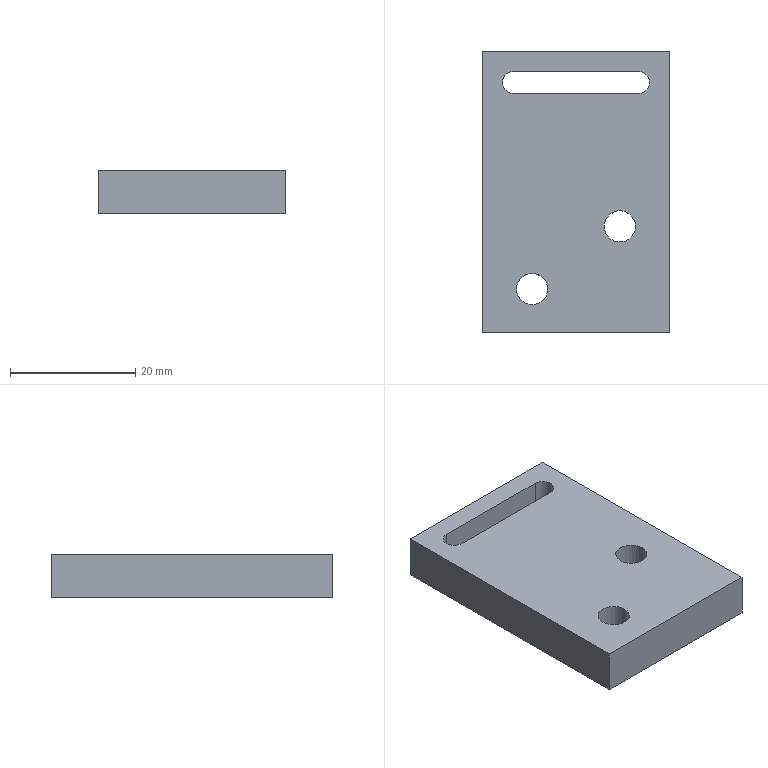Part | SolidWorks | features Cut 1, Extrusion 1, HoleWzd 1 | 1 solid | 15 faces | box 30 x 45 x 7 mm | volume 8618 mm3 | plane 8 | cylinder 7 | commonest cylinder face diameters 5 x4 3.5 x3
STEP:
#1=CARTESIAN_POINT('',(-4.5,-15.5,7.));
#2=VERTEX_POINT('',#1);
#3=CARTESIAN_POINT('',(-9.5,-15.5,7.));
#4=VERTEX_POINT('',#3);
#5=CARTESIAN_POINT('',(-7.,-15.5,7.));
#6=DIRECTION('',(0.,0.,-1.));
#7=DIRECTION('',(-1.,0.,0.));
#8=AXIS2_PLACEMENT_3D('',#5,#6,#7);
#9=CIRCLE('',#8,2.5);
#10=EDGE_CURVE('',#2,#4,#9,.T.);
#11=ORIENTED_EDGE('',*,*,#10,.F.);
#12=CARTESIAN_POINT('',(-4.5,-15.5,0.));
#13=VERTEX_POINT('',#12);
#14=CARTESIAN_POINT('',(-4.5,-15.5,0.));
#15=DIRECTION('',(0.,0.,-1.));
#16=VECTOR('',#15,1000.);
#17=LINE('',#14,#16);
#18=EDGE_CURVE('',#2,#13,#17,.T.);
#19=ORIENTED_EDGE('',*,*,#18,.T.);
#20=CARTESIAN_POINT('',(-9.5,-15.5,0.));
#21=VERTEX_POINT('',#20);
#22=CARTESIAN_POINT('',(-7.,-15.5,0.));
#23=DIRECTION('',(0.,0.,-1.));
#24=DIRECTION('',(-1.,0.,0.));
#25=AXIS2_PLACEMENT_3D('',#22,#23,#24);
#26=CIRCLE('',#25,2.5);
#27=EDGE_CURVE('',#13,#21,#26,.T.);
#28=ORIENTED_EDGE('',*,*,#27,.T.);
#29=CARTESIAN_POINT('',(-9.5,-15.5,0.));
#30=DIRECTION('',(0.,0.,-1.));
#31=VECTOR('',#30,1000.);
#32=LINE('',#29,#31);
#33=EDGE_CURVE('',#4,#21,#32,.T.);
#34=ORIENTED_EDGE('',*,*,#33,.F.);
#35=EDGE_LOOP('',(#11,#19,#28,#34));
#36=FACE_OUTER_BOUND('',#35,.T.);
#37=CARTESIAN_POINT('',(-7.,-15.5,0.));
#38=DIRECTION('',(0.,0.,-1.));
#39=DIRECTION('',(-1.,0.,0.));
#40=AXIS2_PLACEMENT_3D('',#37,#38,#39);
#41=CYLINDRICAL_SURFACE('',#40,2.5);
#42=ADVANCED_FACE('',(#36),#41,.F.);
#43=CARTESIAN_POINT('',(9.5,-5.5,7.));
#44=VERTEX_POINT('',#43);
#45=CARTESIAN_POINT('',(4.5,-5.5,7.));
#46=VERTEX_POINT('',#45);
#47=CARTESIAN_POINT('',(7.,-5.5,7.));
#48=DIRECTION('',(0.,0.,-1.));
#49=DIRECTION('',(-1.,0.,0.));
#50=AXIS2_PLACEMENT_3D('',#47,#48,#49);
#51=CIRCLE('',#50,2.5);
#52=EDGE_CURVE('',#44,#46,#51,.T.);
#53=ORIENTED_EDGE('',*,*,#52,.F.);
#54=CARTESIAN_POINT('',(9.5,-5.5,0.));
#55=VERTEX_POINT('',#54);
#56=CARTESIAN_POINT('',(9.5,-5.5,0.));
#57=DIRECTION('',(0.,0.,-1.));
#58=VECTOR('',#57,1000.);
#59=LINE('',#56,#58);
#60=EDGE_CURVE('',#44,#55,#59,.T.);
#61=ORIENTED_EDGE('',*,*,#60,.T.);
#62=CARTESIAN_POINT('',(4.5,-5.5,0.));
#63=VERTEX_POINT('',#62);
#64=CARTESIAN_POINT('',(7.,-5.5,0.));
#65=DIRECTION('',(0.,0.,-1.));
#66=DIRECTION('',(-1.,0.,0.));
#67=AXIS2_PLACEMENT_3D('',#64,#65,#66);
#68=CIRCLE('',#67,2.5);
#69=EDGE_CURVE('',#55,#63,#68,.T.);
#70=ORIENTED_EDGE('',*,*,#69,.T.);
#71=CARTESIAN_POINT('',(4.5,-5.5,0.));
#72=DIRECTION('',(0.,0.,-1.));
#73=VECTOR('',#72,1000.);
#74=LINE('',#71,#73);
#75=EDGE_CURVE('',#46,#63,#74,.T.);
#76=ORIENTED_EDGE('',*,*,#75,.F.);
#77=EDGE_LOOP('',(#53,#61,#70,#76));
#78=FACE_OUTER_BOUND('',#77,.T.);
#79=CARTESIAN_POINT('',(7.,-5.5,0.));
#80=DIRECTION('',(0.,0.,-1.));
#81=DIRECTION('',(-1.,0.,0.));
#82=AXIS2_PLACEMENT_3D('',#79,#80,#81);
#83=CYLINDRICAL_SURFACE('',#82,2.5);
#84=ADVANCED_FACE('',(#78),#83,.F.);
#85=CARTESIAN_POINT('',(-11.75,17.5,7.));
#86=VERTEX_POINT('',#85);
#87=CARTESIAN_POINT('',(-10.,19.25,7.));
#88=VERTEX_POINT('',#87);
#89=CARTESIAN_POINT('',(-10.,17.5,7.));
#90=DIRECTION('',(0.,0.,-1.));
#91=DIRECTION('',(-1.,0.,0.));
#92=AXIS2_PLACEMENT_3D('',#89,#90,#91);
#93=CIRCLE('',#92,1.75);
#94=EDGE_CURVE('',#86,#88,#93,.T.);
#95=ORIENTED_EDGE('',*,*,#94,.F.);
#96=CARTESIAN_POINT('',(-11.75,17.5,0.));
#97=VERTEX_POINT('',#96);
#98=CARTESIAN_POINT('',(-11.75,17.5,7.));
#99=DIRECTION('',(0.,0.,-1.));
#100=VECTOR('',#99,1000.);
#101=LINE('',#98,#100);
#102=EDGE_CURVE('',#86,#97,#101,.T.);
#103=ORIENTED_EDGE('',*,*,#102,.T.);
#104=CARTESIAN_POINT('',(-10.,19.25,0.));
#105=VERTEX_POINT('',#104);
#106=CARTESIAN_POINT('',(-10.,17.5,0.));
#107=DIRECTION('',(0.,0.,-1.));
#108=DIRECTION('',(-1.,0.,0.));
#109=AXIS2_PLACEMENT_3D('',#106,#107,#108);
#110=CIRCLE('',#109,1.75);
#111=EDGE_CURVE('',#97,#105,#110,.T.);
#112=ORIENTED_EDGE('',*,*,#111,.T.);
#113=CARTESIAN_POINT('',(-10.,19.25,7.));
#114=DIRECTION('',(0.,0.,-1.));
#115=VECTOR('',#114,1000.);
#116=LINE('',#113,#115);
#117=EDGE_CURVE('',#88,#105,#116,.T.);
#118=ORIENTED_EDGE('',*,*,#117,.F.);
#119=EDGE_LOOP('',(#95,#103,#112,#118));
#120=FACE_OUTER_BOUND('',#119,.T.);
#121=CARTESIAN_POINT('',(-10.,17.5,7.));
#122=DIRECTION('',(0.,0.,-1.));
#123=DIRECTION('',(-1.,0.,0.));
#124=AXIS2_PLACEMENT_3D('',#121,#122,#123);
#125=CYLINDRICAL_SURFACE('',#124,1.75);
#126=ADVANCED_FACE('',(#120),#125,.F.);
#127=CARTESIAN_POINT('',(15.,-22.5,0.));
#128=VERTEX_POINT('',#127);
#129=CARTESIAN_POINT('',(15.,22.5,0.));
#130=VERTEX_POINT('',#129);
#131=CARTESIAN_POINT('',(15.,-22.5,0.));
#132=DIRECTION('',(0.,1.,0.));
#133=VECTOR('',#132,1000.);
#134=LINE('',#131,#133);
#135=EDGE_CURVE('',#128,#130,#134,.T.);
#136=ORIENTED_EDGE('',*,*,#135,.T.);
#137=CARTESIAN_POINT('',(15.,22.5,7.));
#138=VERTEX_POINT('',#137);
#139=CARTESIAN_POINT('',(15.,22.5,7.));
#140=DIRECTION('',(0.,0.,-1.));
#141=VECTOR('',#140,1000.);
#142=LINE('',#139,#141);
#143=EDGE_CURVE('',#138,#130,#142,.T.);
#144=ORIENTED_EDGE('',*,*,#143,.F.);
#145=CARTESIAN_POINT('',(15.,-22.5,7.));
#146=VERTEX_POINT('',#145);
#147=CARTESIAN_POINT('',(15.,-22.5,7.));
#148=DIRECTION('',(0.,1.,0.));
#149=VECTOR('',#148,1000.);
#150=LINE('',#147,#149);
#151=EDGE_CURVE('',#146,#138,#150,.T.);
#152=ORIENTED_EDGE('',*,*,#151,.F.);
#153=CARTESIAN_POINT('',(15.,-22.5,7.));
#154=DIRECTION('',(0.,0.,-1.));
#155=VECTOR('',#154,1000.);
#156=LINE('',#153,#155);
#157=EDGE_CURVE('',#146,#128,#156,.T.);
#158=ORIENTED_EDGE('',*,*,#157,.T.);
#159=EDGE_LOOP('',(#136,#144,#152,#158));
#160=FACE_OUTER_BOUND('',#159,.T.);
#161=CARTESIAN_POINT('',(15.,-22.5,7.));
#162=DIRECTION('',(-1.,0.,0.));
#163=DIRECTION('',(0.,0.,1.));
#164=AXIS2_PLACEMENT_3D('',#161,#162,#163);
#165=PLANE('',#164);
#166=ADVANCED_FACE('',(#160),#165,.F.);
#167=CARTESIAN_POINT('',(-15.,22.5,0.));
#168=VERTEX_POINT('',#167);
#169=CARTESIAN_POINT('',(-15.,22.5,0.));
#170=DIRECTION('',(-1.,0.,0.));
#171=VECTOR('',#170,1000.);
#172=LINE('',#169,#171);
#173=EDGE_CURVE('',#130,#168,#172,.T.);
#174=ORIENTED_EDGE('',*,*,#173,.T.);
#175=CARTESIAN_POINT('',(-15.,22.5,7.));
#176=VERTEX_POINT('',#175);
#177=CARTESIAN_POINT('',(-15.,22.5,7.));
#178=DIRECTION('',(0.,0.,-1.));
#179=VECTOR('',#178,1000.);
#180=LINE('',#177,#179);
#181=EDGE_CURVE('',#176,#168,#180,.T.);
#182=ORIENTED_EDGE('',*,*,#181,.F.);
#183=CARTESIAN_POINT('',(-15.,22.5,7.));
#184=DIRECTION('',(-1.,0.,0.));
#185=VECTOR('',#184,1000.);
#186=LINE('',#183,#185);
#187=EDGE_CURVE('',#138,#176,#186,.T.);
#188=ORIENTED_EDGE('',*,*,#187,.F.);
#189=ORIENTED_EDGE('',*,*,#143,.T.);
#190=EDGE_LOOP('',(#174,#182,#188,#189));
#191=FACE_OUTER_BOUND('',#190,.T.);
#192=CARTESIAN_POINT('',(-15.,22.5,7.));
#193=DIRECTION('',(0.,-1.,0.));
#194=DIRECTION('',(0.,0.,-1.));
#195=AXIS2_PLACEMENT_3D('',#192,#193,#194);
#196=PLANE('',#195);
#197=ADVANCED_FACE('',(#191),#196,.F.);
#198=CARTESIAN_POINT('',(-15.,-22.5,0.));
#199=VERTEX_POINT('',#198);
#200=CARTESIAN_POINT('',(-15.,-22.5,0.));
#201=DIRECTION('',(0.,-1.,0.));
#202=VECTOR('',#201,1000.);
#203=LINE('',#200,#202);
#204=EDGE_CURVE('',#168,#199,#203,.T.);
#205=ORIENTED_EDGE('',*,*,#204,.T.);
#206=CARTESIAN_POINT('',(-15.,-22.5,7.));
#207=VERTEX_POINT('',#206);
#208=CARTESIAN_POINT('',(-15.,-22.5,7.));
#209=DIRECTION('',(0.,0.,-1.));
#210=VECTOR('',#209,1000.);
#211=LINE('',#208,#210);
#212=EDGE_CURVE('',#207,#199,#211,.T.);
#213=ORIENTED_EDGE('',*,*,#212,.F.);
#214=CARTESIAN_POINT('',(-15.,-22.5,7.));
#215=DIRECTION('',(0.,-1.,0.));
#216=VECTOR('',#215,1000.);
#217=LINE('',#214,#216);
#218=EDGE_CURVE('',#176,#207,#217,.T.);
#219=ORIENTED_EDGE('',*,*,#218,.F.);
#220=ORIENTED_EDGE('',*,*,#181,.T.);
#221=EDGE_LOOP('',(#205,#213,#219,#220));
#222=FACE_OUTER_BOUND('',#221,.T.);
#223=CARTESIAN_POINT('',(-15.,-22.5,7.));
#224=DIRECTION('',(1.,0.,0.));
#225=DIRECTION('',(0.,0.,-1.));
#226=AXIS2_PLACEMENT_3D('',#223,#224,#225);
#227=PLANE('',#226);
#228=ADVANCED_FACE('',(#222),#227,.F.);
#229=CARTESIAN_POINT('',(-15.,-22.5,0.));
#230=DIRECTION('',(1.,0.,0.));
#231=VECTOR('',#230,1000.);
#232=LINE('',#229,#231);
#233=EDGE_CURVE('',#199,#128,#232,.T.);
#234=ORIENTED_EDGE('',*,*,#233,.T.);
#235=ORIENTED_EDGE('',*,*,#157,.F.);
#236=CARTESIAN_POINT('',(-15.,-22.5,7.));
#237=DIRECTION('',(1.,0.,0.));
#238=VECTOR('',#237,1000.);
#239=LINE('',#236,#238);
#240=EDGE_CURVE('',#207,#146,#239,.T.);
#241=ORIENTED_EDGE('',*,*,#240,.F.);
#242=ORIENTED_EDGE('',*,*,#212,.T.);
#243=EDGE_LOOP('',(#234,#235,#241,#242));
#244=FACE_OUTER_BOUND('',#243,.T.);
#245=CARTESIAN_POINT('',(-15.,-22.5,7.));
#246=DIRECTION('',(0.,1.,0.));
#247=DIRECTION('',(0.,0.,1.));
#248=AXIS2_PLACEMENT_3D('',#245,#246,#247);
#249=PLANE('',#248);
#250=ADVANCED_FACE('',(#244),#249,.F.);
#251=CARTESIAN_POINT('',(-7.,-15.5,7.));
#252=DIRECTION('',(0.,0.,-1.));
#253=DIRECTION('',(-1.,0.,0.));
#254=AXIS2_PLACEMENT_3D('',#251,#252,#253);
#255=CIRCLE('',#254,2.5);
#256=EDGE_CURVE('',#4,#2,#255,.T.);
#257=ORIENTED_EDGE('',*,*,#256,.T.);
#258=ORIENTED_EDGE('',*,*,#10,.T.);
#259=EDGE_LOOP('',(#257,#258));
#260=FACE_BOUND('',#259,.T.);
#261=CARTESIAN_POINT('',(7.,-5.5,7.));
#262=DIRECTION('',(0.,0.,-1.));
#263=DIRECTION('',(-1.,0.,0.));
#264=AXIS2_PLACEMENT_3D('',#261,#262,#263);
#265=CIRCLE('',#264,2.5);
#266=EDGE_CURVE('',#46,#44,#265,.T.);
#267=ORIENTED_EDGE('',*,*,#266,.T.);
#268=ORIENTED_EDGE('',*,*,#52,.T.);
#269=EDGE_LOOP('',(#267,#268));
#270=FACE_BOUND('',#269,.T.);
#271=CARTESIAN_POINT('',(10.,15.75,7.));
#272=VERTEX_POINT('',#271);
#273=CARTESIAN_POINT('',(-10.,15.75,7.));
#274=VERTEX_POINT('',#273);
#275=CARTESIAN_POINT('',(-10.,15.75,7.));
#276=DIRECTION('',(-1.,0.,0.));
#277=VECTOR('',#276,1000.);
#278=LINE('',#275,#277);
#279=EDGE_CURVE('',#272,#274,#278,.T.);
#280=ORIENTED_EDGE('',*,*,#279,.T.);
#281=CARTESIAN_POINT('',(-10.,17.5,7.));
#282=DIRECTION('',(0.,0.,-1.));
#283=DIRECTION('',(-1.,0.,0.));
#284=AXIS2_PLACEMENT_3D('',#281,#282,#283);
#285=CIRCLE('',#284,1.75);
#286=EDGE_CURVE('',#274,#86,#285,.T.);
#287=ORIENTED_EDGE('',*,*,#286,.T.);
#288=ORIENTED_EDGE('',*,*,#94,.T.);
#289=CARTESIAN_POINT('',(10.,19.25,7.));
#290=VERTEX_POINT('',#289);
#291=CARTESIAN_POINT('',(-10.,19.25,7.));
#292=DIRECTION('',(1.,0.,0.));
#293=VECTOR('',#292,1000.);
#294=LINE('',#291,#293);
#295=EDGE_CURVE('',#88,#290,#294,.T.);
#296=ORIENTED_EDGE('',*,*,#295,.T.);
#297=CARTESIAN_POINT('',(10.,17.5,7.));
#298=DIRECTION('',(0.,0.,-1.));
#299=DIRECTION('',(-1.,0.,0.));
#300=AXIS2_PLACEMENT_3D('',#297,#298,#299);
#301=CIRCLE('',#300,1.75);
#302=EDGE_CURVE('',#290,#272,#301,.T.);
#303=ORIENTED_EDGE('',*,*,#302,.T.);
#304=EDGE_LOOP('',(#280,#287,#288,#296,#303));
#305=FACE_BOUND('',#304,.T.);
#306=ORIENTED_EDGE('',*,*,#151,.T.);
#307=ORIENTED_EDGE('',*,*,#187,.T.);
#308=ORIENTED_EDGE('',*,*,#218,.T.);
#309=ORIENTED_EDGE('',*,*,#240,.T.);
#310=EDGE_LOOP('',(#306,#307,#308,#309));
#311=FACE_OUTER_BOUND('',#310,.T.);
#312=CARTESIAN_POINT('',(15.,22.5,7.));
#313=DIRECTION('',(0.,0.,-1.));
#314=DIRECTION('',(-1.,0.,0.));
#315=AXIS2_PLACEMENT_3D('',#312,#313,#314);
#316=PLANE('',#315);
#317=ADVANCED_FACE('',(#260,#270,#305,#311),#316,.F.);
#318=CARTESIAN_POINT('',(-7.,-15.5,0.));
#319=DIRECTION('',(0.,0.,-1.));
#320=DIRECTION('',(-1.,0.,0.));
#321=AXIS2_PLACEMENT_3D('',#318,#319,#320);
#322=CIRCLE('',#321,2.5);
#323=EDGE_CURVE('',#21,#13,#322,.T.);
#324=ORIENTED_EDGE('',*,*,#323,.F.);
#325=ORIENTED_EDGE('',*,*,#27,.F.);
#326=EDGE_LOOP('',(#324,#325));
#327=FACE_BOUND('',#326,.T.);
#328=CARTESIAN_POINT('',(7.,-5.5,0.));
#329=DIRECTION('',(0.,0.,-1.));
#330=DIRECTION('',(-1.,0.,0.));
#331=AXIS2_PLACEMENT_3D('',#328,#329,#330);
#332=CIRCLE('',#331,2.5);
#333=EDGE_CURVE('',#63,#55,#332,.T.);
#334=ORIENTED_EDGE('',*,*,#333,.F.);
#335=ORIENTED_EDGE('',*,*,#69,.F.);
#336=EDGE_LOOP('',(#334,#335));
#337=FACE_BOUND('',#336,.T.);
#338=CARTESIAN_POINT('',(-10.,15.75,0.));
#339=VERTEX_POINT('',#338);
#340=CARTESIAN_POINT('',(-10.,17.5,0.));
#341=DIRECTION('',(0.,0.,-1.));
#342=DIRECTION('',(-1.,0.,0.));
#343=AXIS2_PLACEMENT_3D('',#340,#341,#342);
#344=CIRCLE('',#343,1.75);
#345=EDGE_CURVE('',#339,#97,#344,.T.);
#346=ORIENTED_EDGE('',*,*,#345,.F.);
#347=CARTESIAN_POINT('',(10.,15.75,0.));
#348=VERTEX_POINT('',#347);
#349=CARTESIAN_POINT('',(-10.,15.75,0.));
#350=DIRECTION('',(-1.,0.,0.));
#351=VECTOR('',#350,1000.);
#352=LINE('',#349,#351);
#353=EDGE_CURVE('',#348,#339,#352,.T.);
#354=ORIENTED_EDGE('',*,*,#353,.F.);
#355=CARTESIAN_POINT('',(10.,19.25,0.));
#356=VERTEX_POINT('',#355);
#357=CARTESIAN_POINT('',(10.,17.5,0.));
#358=DIRECTION('',(0.,0.,-1.));
#359=DIRECTION('',(-1.,0.,0.));
#360=AXIS2_PLACEMENT_3D('',#357,#358,#359);
#361=CIRCLE('',#360,1.75);
#362=EDGE_CURVE('',#356,#348,#361,.T.);
#363=ORIENTED_EDGE('',*,*,#362,.F.);
#364=CARTESIAN_POINT('',(-10.,19.25,0.));
#365=DIRECTION('',(1.,0.,0.));
#366=VECTOR('',#365,1000.);
#367=LINE('',#364,#366);
#368=EDGE_CURVE('',#105,#356,#367,.T.);
#369=ORIENTED_EDGE('',*,*,#368,.F.);
#370=ORIENTED_EDGE('',*,*,#111,.F.);
#371=EDGE_LOOP('',(#346,#354,#363,#369,#370));
#372=FACE_BOUND('',#371,.T.);
#373=ORIENTED_EDGE('',*,*,#135,.F.);
#374=ORIENTED_EDGE('',*,*,#233,.F.);
#375=ORIENTED_EDGE('',*,*,#204,.F.);
#376=ORIENTED_EDGE('',*,*,#173,.F.);
#377=EDGE_LOOP('',(#373,#374,#375,#376));
#378=FACE_OUTER_BOUND('',#377,.T.);
#379=CARTESIAN_POINT('',(15.,22.5,0.));
#380=DIRECTION('',(0.,0.,-1.));
#381=DIRECTION('',(-1.,0.,0.));
#382=AXIS2_PLACEMENT_3D('',#379,#380,#381);
#383=PLANE('',#382);
#384=ADVANCED_FACE('',(#327,#337,#372,#378),#383,.T.);
#385=ORIENTED_EDGE('',*,*,#102,.F.);
#386=ORIENTED_EDGE('',*,*,#286,.F.);
#387=CARTESIAN_POINT('',(-10.,15.75,7.));
#388=DIRECTION('',(0.,0.,-1.));
#389=VECTOR('',#388,1000.);
#390=LINE('',#387,#389);
#391=EDGE_CURVE('',#274,#339,#390,.T.);
#392=ORIENTED_EDGE('',*,*,#391,.T.);
#393=ORIENTED_EDGE('',*,*,#345,.T.);
#394=EDGE_LOOP('',(#385,#386,#392,#393));
#395=FACE_OUTER_BOUND('',#394,.T.);
#396=CARTESIAN_POINT('',(-10.,17.5,7.));
#397=DIRECTION('',(0.,0.,-1.));
#398=DIRECTION('',(-1.,0.,0.));
#399=AXIS2_PLACEMENT_3D('',#396,#397,#398);
#400=CYLINDRICAL_SURFACE('',#399,1.75);
#401=ADVANCED_FACE('',(#395),#400,.F.);
#402=ORIENTED_EDGE('',*,*,#353,.T.);
#403=ORIENTED_EDGE('',*,*,#391,.F.);
#404=ORIENTED_EDGE('',*,*,#279,.F.);
#405=CARTESIAN_POINT('',(10.,15.75,7.));
#406=DIRECTION('',(0.,0.,-1.));
#407=VECTOR('',#406,1000.);
#408=LINE('',#405,#407);
#409=EDGE_CURVE('',#272,#348,#408,.T.);
#410=ORIENTED_EDGE('',*,*,#409,.T.);
#411=EDGE_LOOP('',(#402,#403,#404,#410));
#412=FACE_OUTER_BOUND('',#411,.T.);
#413=CARTESIAN_POINT('',(-10.,15.75,7.));
#414=DIRECTION('',(0.,-1.,0.));
#415=DIRECTION('',(1.,0.,0.));
#416=AXIS2_PLACEMENT_3D('',#413,#414,#415);
#417=PLANE('',#416);
#418=ADVANCED_FACE('',(#412),#417,.F.);
#419=ORIENTED_EDGE('',*,*,#362,.T.);
#420=ORIENTED_EDGE('',*,*,#409,.F.);
#421=ORIENTED_EDGE('',*,*,#302,.F.);
#422=CARTESIAN_POINT('',(10.,19.25,7.));
#423=DIRECTION('',(0.,0.,-1.));
#424=VECTOR('',#423,1000.);
#425=LINE('',#422,#424);
#426=EDGE_CURVE('',#290,#356,#425,.T.);
#427=ORIENTED_EDGE('',*,*,#426,.T.);
#428=EDGE_LOOP('',(#419,#420,#421,#427));
#429=FACE_OUTER_BOUND('',#428,.T.);
#430=CARTESIAN_POINT('',(10.,17.5,7.));
#431=DIRECTION('',(0.,0.,-1.));
#432=DIRECTION('',(-1.,0.,0.));
#433=AXIS2_PLACEMENT_3D('',#430,#431,#432);
#434=CYLINDRICAL_SURFACE('',#433,1.75);
#435=ADVANCED_FACE('',(#429),#434,.F.);
#436=ORIENTED_EDGE('',*,*,#368,.T.);
#437=ORIENTED_EDGE('',*,*,#426,.F.);
#438=ORIENTED_EDGE('',*,*,#295,.F.);
#439=ORIENTED_EDGE('',*,*,#117,.T.);
#440=EDGE_LOOP('',(#436,#437,#438,#439));
#441=FACE_OUTER_BOUND('',#440,.T.);
#442=CARTESIAN_POINT('',(-10.,19.25,7.));
#443=DIRECTION('',(0.,1.,0.));
#444=DIRECTION('',(-1.,0.,0.));
#445=AXIS2_PLACEMENT_3D('',#442,#443,#444);
#446=PLANE('',#445);
#447=ADVANCED_FACE('',(#441),#446,.F.);
#448=ORIENTED_EDGE('',*,*,#60,.F.);
#449=ORIENTED_EDGE('',*,*,#266,.F.);
#450=ORIENTED_EDGE('',*,*,#75,.T.);
#451=ORIENTED_EDGE('',*,*,#333,.T.);
#452=EDGE_LOOP('',(#448,#449,#450,#451));
#453=FACE_OUTER_BOUND('',#452,.T.);
#454=CARTESIAN_POINT('',(7.,-5.5,0.));
#455=DIRECTION('',(0.,0.,-1.));
#456=DIRECTION('',(-1.,0.,0.));
#457=AXIS2_PLACEMENT_3D('',#454,#455,#456);
#458=CYLINDRICAL_SURFACE('',#457,2.5);
#459=ADVANCED_FACE('',(#453),#458,.F.);
#460=ORIENTED_EDGE('',*,*,#18,.F.);
#461=ORIENTED_EDGE('',*,*,#256,.F.);
#462=ORIENTED_EDGE('',*,*,#33,.T.);
#463=ORIENTED_EDGE('',*,*,#323,.T.);
#464=EDGE_LOOP('',(#460,#461,#462,#463));
#465=FACE_OUTER_BOUND('',#464,.T.);
#466=CARTESIAN_POINT('',(-7.,-15.5,0.));
#467=DIRECTION('',(0.,0.,-1.));
#468=DIRECTION('',(-1.,0.,0.));
#469=AXIS2_PLACEMENT_3D('',#466,#467,#468);
#470=CYLINDRICAL_SURFACE('',#469,2.5);
#471=ADVANCED_FACE('',(#465),#470,.F.);
#472=CLOSED_SHELL('',(#42,#84,#126,#166,#197,#228,#250,#317,#384,#401,#418,#435,#447,#459,#471));
#473=MANIFOLD_SOLID_BREP('',#472);
#474=CARTESIAN_POINT('',(0.,0.,0.));
#475=DIRECTION('',(0.,0.,1.));
#476=DIRECTION('',(1.,0.,0.));
#477=AXIS2_PLACEMENT_3D('',#474,#475,#476);
#478=(LENGTH_UNIT()NAMED_UNIT(*)SI_UNIT(.MILLI.,.METRE.));
#479=UNCERTAINTY_MEASURE_WITH_UNIT(LENGTH_MEASURE(0.00001),#478,'','');
#480=(NAMED_UNIT(*)PLANE_ANGLE_UNIT()SI_UNIT($,.RADIAN.));
#481=(NAMED_UNIT(*)SI_UNIT($,.STERADIAN.)SOLID_ANGLE_UNIT());
#482=(GEOMETRIC_REPRESENTATION_CONTEXT(3)GLOBAL_UNCERTAINTY_ASSIGNED_CONTEXT((#479))GLOBAL_UNIT_ASSIGNED_CONTEXT((#478,#480,#481))REPRESENTATION_CONTEXT('',''));
#483=ADVANCED_BREP_SHAPE_REPRESENTATION('',(#473,#477),#482);